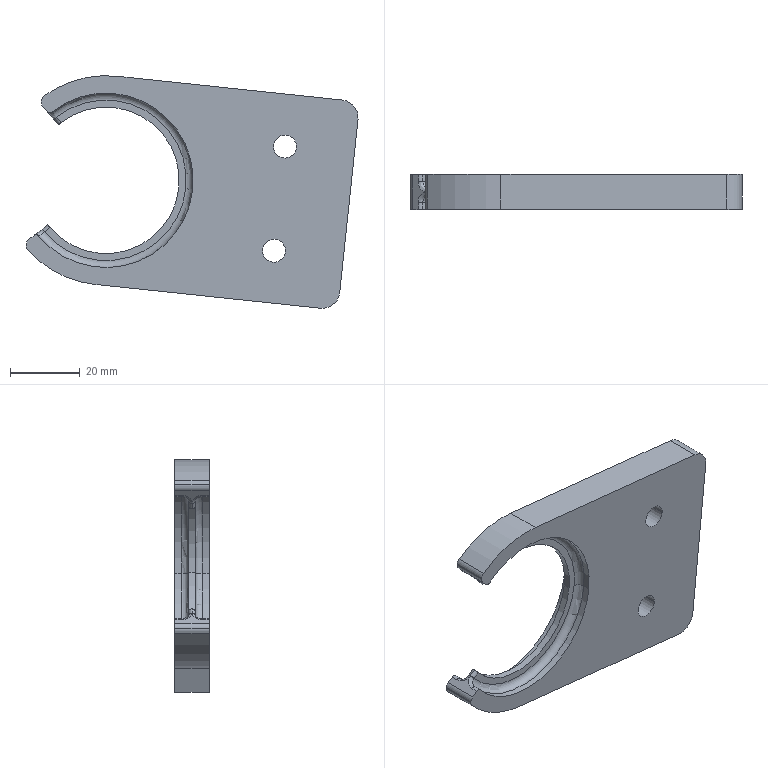Part | STEP file | Fillet 5-6 | 1 solid | 49 faces | box 95.204 x 10 x 66.687 mm | volume 33577 mm3 | cylinder 30 | plane 11 | torus 4 | spline 4 | commonest cylinder face diameters 2 x8 4 x4 6.6 x4 14.55 x4 50 x4 10 x2